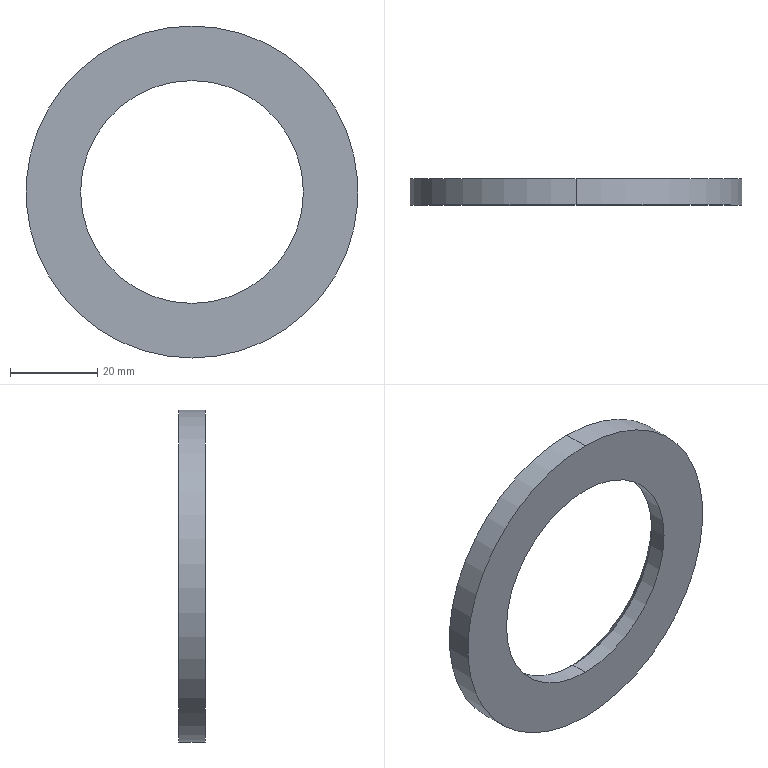Part | SolidWorks | features Chamfer 1, FlatPattern 1, SMBaseFlange 1, SheetMetal 1 | 1 solid | 8 faces | box 76 x 6 x 76 mm | volume 14633 mm3 | cylinder 4 | cone 2 | plane 2 | commonest cylinder face diameters 51 x2 76 x2
STEP:
#1=CARTESIAN_POINT('',(0.,-2.,-25.5));
#2=VERTEX_POINT('',#1);
#3=CARTESIAN_POINT('',(0.,-2.,25.5));
#4=VERTEX_POINT('',#3);
#5=CARTESIAN_POINT('',(0.,-2.,0.));
#6=DIRECTION('',(0.,1.,0.));
#7=DIRECTION('',(0.,0.,1.));
#8=AXIS2_PLACEMENT_3D('',#5,#6,#7);
#9=CIRCLE('',#8,25.5);
#10=EDGE_CURVE('',#2,#4,#9,.T.);
#11=ORIENTED_EDGE('',*,*,#10,.F.);
#12=CARTESIAN_POINT('',(0.,0.,-27.5));
#13=VERTEX_POINT('',#12);
#14=CARTESIAN_POINT('',(0.,-2.,-25.5));
#15=DIRECTION('',(0.,0.7071,-0.7071));
#16=VECTOR('',#15,1000.);
#17=LINE('',#14,#16);
#18=EDGE_CURVE('',#2,#13,#17,.T.);
#19=ORIENTED_EDGE('',*,*,#18,.T.);
#20=CARTESIAN_POINT('',(0.,0.,27.5));
#21=VERTEX_POINT('',#20);
#22=CARTESIAN_POINT('',(0.,0.,0.));
#23=DIRECTION('',(0.,-1.,0.));
#24=DIRECTION('',(0.,0.,1.));
#25=AXIS2_PLACEMENT_3D('',#22,#23,#24);
#26=CIRCLE('',#25,27.5);
#27=EDGE_CURVE('',#21,#13,#26,.T.);
#28=ORIENTED_EDGE('',*,*,#27,.F.);
#29=CARTESIAN_POINT('',(0.,-2.,25.5));
#30=DIRECTION('',(0.,0.7071,0.7071));
#31=VECTOR('',#30,1000.);
#32=LINE('',#29,#31);
#33=EDGE_CURVE('',#4,#21,#32,.T.);
#34=ORIENTED_EDGE('',*,*,#33,.F.);
#35=EDGE_LOOP('',(#11,#19,#28,#34));
#36=FACE_OUTER_BOUND('',#35,.T.);
#37=CARTESIAN_POINT('',(0.,-2.,0.));
#38=DIRECTION('',(0.,1.,0.));
#39=DIRECTION('',(0.,0.,1.));
#40=AXIS2_PLACEMENT_3D('',#37,#38,#39);
#41=CONICAL_SURFACE('',#40,25.5,0.7854);
#42=ADVANCED_FACE('',(#36),#41,.F.);
#43=CARTESIAN_POINT('',(0.,-6.,-25.5));
#44=VERTEX_POINT('',#43);
#45=CARTESIAN_POINT('',(0.,-6.,25.5));
#46=VERTEX_POINT('',#45);
#47=CARTESIAN_POINT('',(0.,-6.,0.));
#48=DIRECTION('',(0.,1.,0.));
#49=DIRECTION('',(0.,0.,1.));
#50=AXIS2_PLACEMENT_3D('',#47,#48,#49);
#51=CIRCLE('',#50,25.5);
#52=EDGE_CURVE('',#44,#46,#51,.T.);
#53=ORIENTED_EDGE('',*,*,#52,.F.);
#54=CARTESIAN_POINT('',(0.,-6.,-25.5));
#55=DIRECTION('',(0.,1.,0.));
#56=VECTOR('',#55,1000.);
#57=LINE('',#54,#56);
#58=EDGE_CURVE('',#44,#2,#57,.T.);
#59=ORIENTED_EDGE('',*,*,#58,.T.);
#60=ORIENTED_EDGE('',*,*,#10,.T.);
#61=CARTESIAN_POINT('',(0.,-6.,25.5));
#62=DIRECTION('',(0.,1.,0.));
#63=VECTOR('',#62,1000.);
#64=LINE('',#61,#63);
#65=EDGE_CURVE('',#46,#4,#64,.T.);
#66=ORIENTED_EDGE('',*,*,#65,.F.);
#67=EDGE_LOOP('',(#53,#59,#60,#66));
#68=FACE_OUTER_BOUND('',#67,.T.);
#69=CARTESIAN_POINT('',(0.,-6.,0.));
#70=DIRECTION('',(0.,1.,0.));
#71=DIRECTION('',(0.,0.,1.));
#72=AXIS2_PLACEMENT_3D('',#69,#70,#71);
#73=CYLINDRICAL_SURFACE('',#72,25.5);
#74=ADVANCED_FACE('',(#68),#73,.F.);
#75=CARTESIAN_POINT('',(0.,-6.,38.));
#76=VERTEX_POINT('',#75);
#77=CARTESIAN_POINT('',(0.,-6.,-38.));
#78=VERTEX_POINT('',#77);
#79=CARTESIAN_POINT('',(0.,-6.,0.));
#80=DIRECTION('',(0.,1.,0.));
#81=DIRECTION('',(0.,0.,1.));
#82=AXIS2_PLACEMENT_3D('',#79,#80,#81);
#83=CIRCLE('',#82,38.);
#84=EDGE_CURVE('',#76,#78,#83,.T.);
#85=ORIENTED_EDGE('',*,*,#84,.T.);
#86=CARTESIAN_POINT('',(0.,0.,-38.));
#87=VERTEX_POINT('',#86);
#88=CARTESIAN_POINT('',(0.,-6.,-38.));
#89=DIRECTION('',(0.,1.,0.));
#90=VECTOR('',#89,1000.);
#91=LINE('',#88,#90);
#92=EDGE_CURVE('',#78,#87,#91,.T.);
#93=ORIENTED_EDGE('',*,*,#92,.T.);
#94=CARTESIAN_POINT('',(0.,0.,38.));
#95=VERTEX_POINT('',#94);
#96=CARTESIAN_POINT('',(0.,0.,0.));
#97=DIRECTION('',(0.,1.,0.));
#98=DIRECTION('',(0.,0.,1.));
#99=AXIS2_PLACEMENT_3D('',#96,#97,#98);
#100=CIRCLE('',#99,38.);
#101=EDGE_CURVE('',#95,#87,#100,.T.);
#102=ORIENTED_EDGE('',*,*,#101,.F.);
#103=CARTESIAN_POINT('',(0.,-6.,38.));
#104=DIRECTION('',(0.,1.,0.));
#105=VECTOR('',#104,1000.);
#106=LINE('',#103,#105);
#107=EDGE_CURVE('',#76,#95,#106,.T.);
#108=ORIENTED_EDGE('',*,*,#107,.F.);
#109=EDGE_LOOP('',(#85,#93,#102,#108));
#110=FACE_OUTER_BOUND('',#109,.T.);
#111=CARTESIAN_POINT('',(0.,-6.,0.));
#112=DIRECTION('',(0.,1.,0.));
#113=DIRECTION('',(0.,0.,1.));
#114=AXIS2_PLACEMENT_3D('',#111,#112,#113);
#115=CYLINDRICAL_SURFACE('',#114,38.);
#116=ADVANCED_FACE('',(#110),#115,.T.);
#117=ORIENTED_EDGE('',*,*,#92,.F.);
#118=CARTESIAN_POINT('',(0.,-6.,0.));
#119=DIRECTION('',(0.,1.,0.));
#120=DIRECTION('',(0.,0.,1.));
#121=AXIS2_PLACEMENT_3D('',#118,#119,#120);
#122=CIRCLE('',#121,38.);
#123=EDGE_CURVE('',#78,#76,#122,.T.);
#124=ORIENTED_EDGE('',*,*,#123,.T.);
#125=ORIENTED_EDGE('',*,*,#107,.T.);
#126=CARTESIAN_POINT('',(0.,0.,0.));
#127=DIRECTION('',(0.,1.,0.));
#128=DIRECTION('',(0.,0.,1.));
#129=AXIS2_PLACEMENT_3D('',#126,#127,#128);
#130=CIRCLE('',#129,38.);
#131=EDGE_CURVE('',#87,#95,#130,.T.);
#132=ORIENTED_EDGE('',*,*,#131,.F.);
#133=EDGE_LOOP('',(#117,#124,#125,#132));
#134=FACE_OUTER_BOUND('',#133,.T.);
#135=CARTESIAN_POINT('',(0.,-6.,0.));
#136=DIRECTION('',(0.,1.,0.));
#137=DIRECTION('',(0.,0.,1.));
#138=AXIS2_PLACEMENT_3D('',#135,#136,#137);
#139=CYLINDRICAL_SURFACE('',#138,38.);
#140=ADVANCED_FACE('',(#134),#139,.T.);
#141=CARTESIAN_POINT('',(0.,-6.,0.));
#142=DIRECTION('',(0.,1.,0.));
#143=DIRECTION('',(0.,0.,1.));
#144=AXIS2_PLACEMENT_3D('',#141,#142,#143);
#145=CIRCLE('',#144,25.5);
#146=EDGE_CURVE('',#46,#44,#145,.T.);
#147=ORIENTED_EDGE('',*,*,#146,.T.);
#148=ORIENTED_EDGE('',*,*,#52,.T.);
#149=EDGE_LOOP('',(#147,#148));
#150=FACE_BOUND('',#149,.T.);
#151=ORIENTED_EDGE('',*,*,#84,.F.);
#152=ORIENTED_EDGE('',*,*,#123,.F.);
#153=EDGE_LOOP('',(#151,#152));
#154=FACE_OUTER_BOUND('',#153,.T.);
#155=CARTESIAN_POINT('',(0.,-6.,0.));
#156=DIRECTION('',(0.,1.,0.));
#157=DIRECTION('',(0.,0.,1.));
#158=AXIS2_PLACEMENT_3D('',#155,#156,#157);
#159=PLANE('',#158);
#160=ADVANCED_FACE('',(#150,#154),#159,.F.);
#161=ORIENTED_EDGE('',*,*,#27,.T.);
#162=CARTESIAN_POINT('',(0.,0.,0.));
#163=DIRECTION('',(0.,-1.,0.));
#164=DIRECTION('',(0.,0.,1.));
#165=AXIS2_PLACEMENT_3D('',#162,#163,#164);
#166=CIRCLE('',#165,27.5);
#167=EDGE_CURVE('',#13,#21,#166,.T.);
#168=ORIENTED_EDGE('',*,*,#167,.T.);
#169=EDGE_LOOP('',(#161,#168));
#170=FACE_BOUND('',#169,.T.);
#171=ORIENTED_EDGE('',*,*,#101,.T.);
#172=ORIENTED_EDGE('',*,*,#131,.T.);
#173=EDGE_LOOP('',(#171,#172));
#174=FACE_OUTER_BOUND('',#173,.T.);
#175=CARTESIAN_POINT('',(0.,0.,0.));
#176=DIRECTION('',(0.,1.,0.));
#177=DIRECTION('',(0.,0.,1.));
#178=AXIS2_PLACEMENT_3D('',#175,#176,#177);
#179=PLANE('',#178);
#180=ADVANCED_FACE('',(#170,#174),#179,.T.);
#181=ORIENTED_EDGE('',*,*,#58,.F.);
#182=ORIENTED_EDGE('',*,*,#146,.F.);
#183=ORIENTED_EDGE('',*,*,#65,.T.);
#184=CARTESIAN_POINT('',(0.,-2.,0.));
#185=DIRECTION('',(0.,1.,0.));
#186=DIRECTION('',(0.,0.,1.));
#187=AXIS2_PLACEMENT_3D('',#184,#185,#186);
#188=CIRCLE('',#187,25.5);
#189=EDGE_CURVE('',#4,#2,#188,.T.);
#190=ORIENTED_EDGE('',*,*,#189,.T.);
#191=EDGE_LOOP('',(#181,#182,#183,#190));
#192=FACE_OUTER_BOUND('',#191,.T.);
#193=CARTESIAN_POINT('',(0.,-6.,0.));
#194=DIRECTION('',(0.,1.,0.));
#195=DIRECTION('',(0.,0.,1.));
#196=AXIS2_PLACEMENT_3D('',#193,#194,#195);
#197=CYLINDRICAL_SURFACE('',#196,25.5);
#198=ADVANCED_FACE('',(#192),#197,.F.);
#199=ORIENTED_EDGE('',*,*,#18,.F.);
#200=ORIENTED_EDGE('',*,*,#189,.F.);
#201=ORIENTED_EDGE('',*,*,#33,.T.);
#202=ORIENTED_EDGE('',*,*,#167,.F.);
#203=EDGE_LOOP('',(#199,#200,#201,#202));
#204=FACE_OUTER_BOUND('',#203,.T.);
#205=CARTESIAN_POINT('',(0.,-2.,0.));
#206=DIRECTION('',(0.,1.,0.));
#207=DIRECTION('',(0.,0.,1.));
#208=AXIS2_PLACEMENT_3D('',#205,#206,#207);
#209=CONICAL_SURFACE('',#208,25.5,0.7854);
#210=ADVANCED_FACE('',(#204),#209,.F.);
#211=CLOSED_SHELL('',(#42,#74,#116,#140,#160,#180,#198,#210));
#212=MANIFOLD_SOLID_BREP('',#211);
#213=CARTESIAN_POINT('',(0.,0.,0.));
#214=DIRECTION('',(0.,0.,1.));
#215=DIRECTION('',(1.,0.,0.));
#216=AXIS2_PLACEMENT_3D('',#213,#214,#215);
#217=(LENGTH_UNIT()NAMED_UNIT(*)SI_UNIT(.MILLI.,.METRE.));
#218=UNCERTAINTY_MEASURE_WITH_UNIT(LENGTH_MEASURE(0.00001),#217,'','');
#219=(NAMED_UNIT(*)PLANE_ANGLE_UNIT()SI_UNIT($,.RADIAN.));
#220=(NAMED_UNIT(*)SI_UNIT($,.STERADIAN.)SOLID_ANGLE_UNIT());
#221=(GEOMETRIC_REPRESENTATION_CONTEXT(3)GLOBAL_UNCERTAINTY_ASSIGNED_CONTEXT((#218))GLOBAL_UNIT_ASSIGNED_CONTEXT((#217,#219,#220))REPRESENTATION_CONTEXT('',''));
#222=ADVANCED_BREP_SHAPE_REPRESENTATION('',(#212,#216),#221);